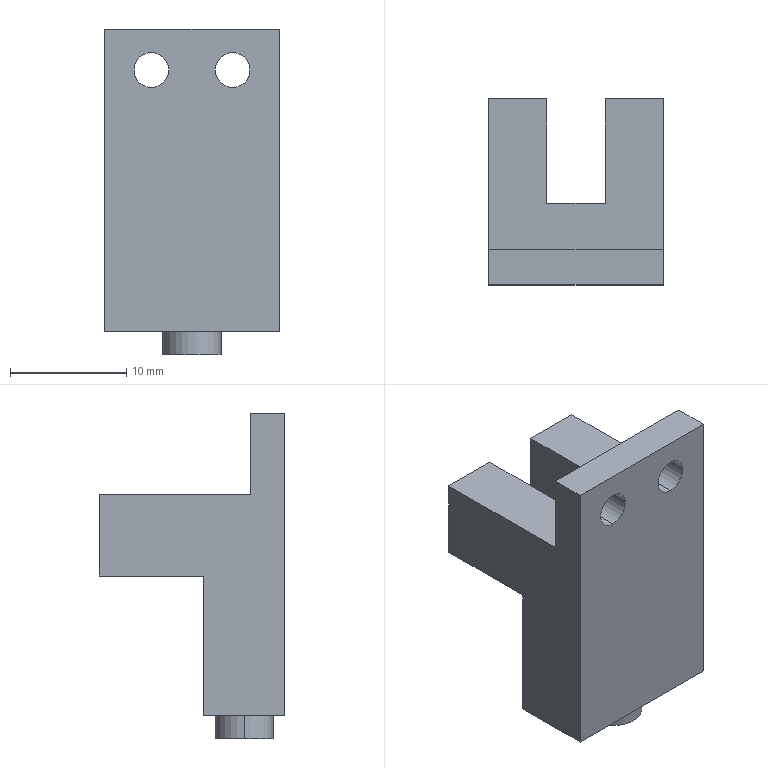Part | STEP file | slot-type photoelectric LU674-5NA | 1 solid | 21 faces | box 15 x 16 x 28 mm | volume 2937 mm3 | plane 15 | cylinder 6 | commonest cylinder face diameters 3 x4 5 x2